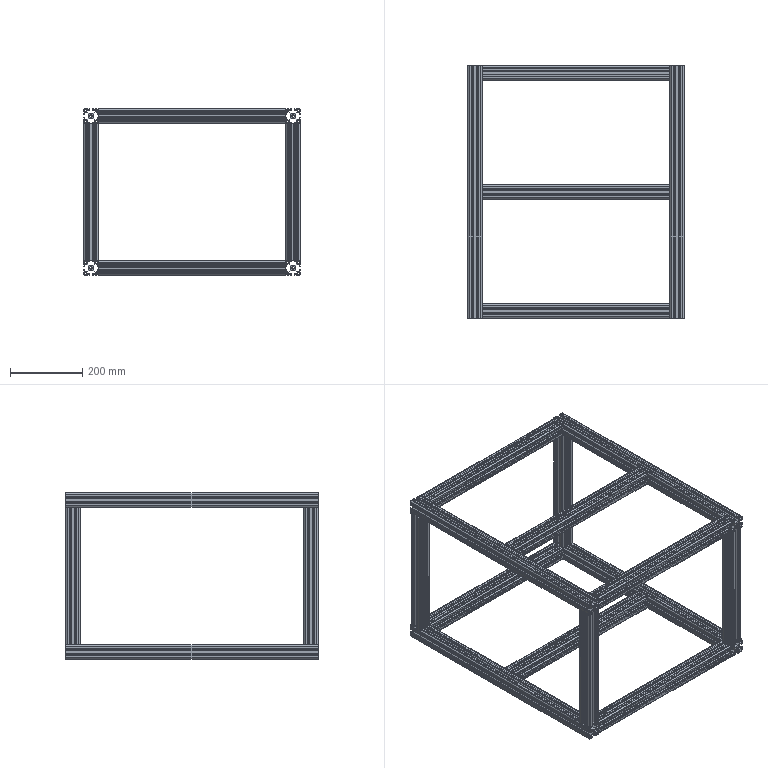Part | STEP file | Grinding bracket-unit 2_Default<machined> | 14 solids | 1456 faces | box 600 x 700 x 460 mm | volume 3532999 mm3 | plane 1316 | cylinder 140 | commonest cylinder face diameters 5 x56 9 x56 6.8 x28